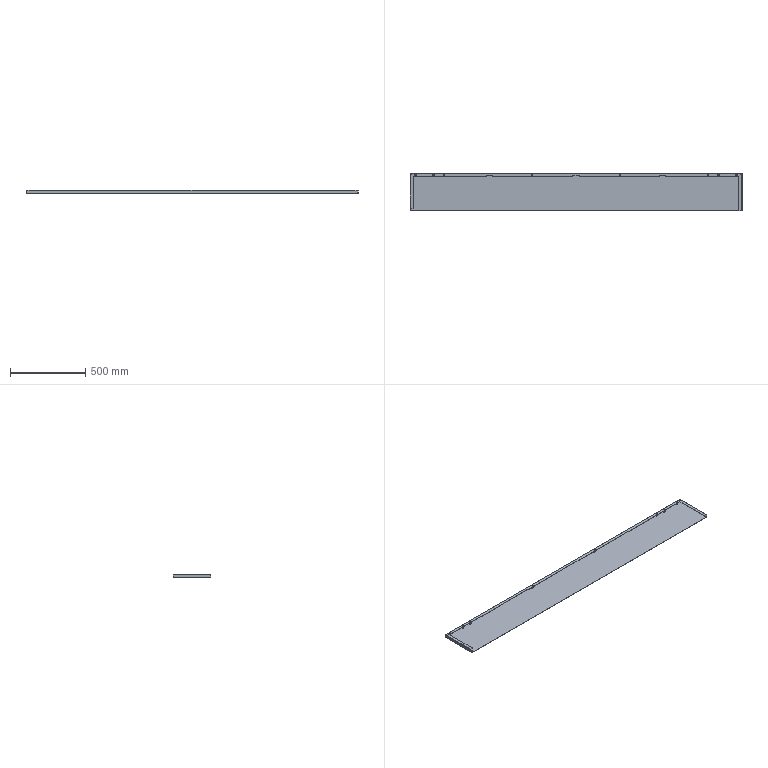Part | SolidWorks | features ICE 6, EdgeFlange 2, MirrorPattern 2, FlatPattern 1, LPattern 1, SMBaseFlange 1, SheetMetal 1 | 1 solid | 126 faces | box 2210 x 251.5 x 20 mm | volume 975971 mm3 | plane 66 | cylinder 52 | spline 8 | commonest cylinder face diameters 6 x24 10 x16 1 x6 4 x6